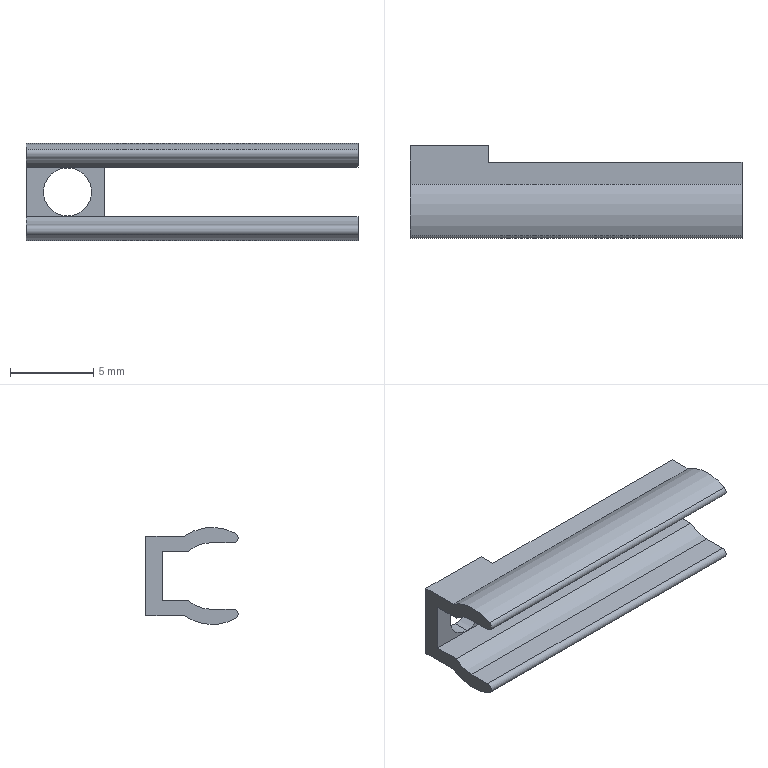Part | SolidWorks | features BaseBody 1 | 1 solid | 23 faces | box 20 x 5.565 x 5.85 mm | volume 175.472 mm3 | plane 14 | cylinder 9 | commonest cylinder face diameters 5.85 x3 0.6 x2 2.9 x2 4 x2
STEP:
#1=CARTESIAN_POINT('',(-0.5,-1.51,-2.563));
#2=VERTEX_POINT('',#1);
#3=CARTESIAN_POINT('',(-0.5,-0.1,-2.925));
#4=VERTEX_POINT('',#3);
#5=CARTESIAN_POINT('',(-0.5,-0.1,0.));
#6=DIRECTION('',(1.,0.,0.));
#7=DIRECTION('',(0.,0.,-1.));
#8=AXIS2_PLACEMENT_3D('',#5,#6,#7);
#9=CIRCLE('',#8,2.925);
#10=EDGE_CURVE('',#2,#4,#9,.T.);
#11=ORIENTED_EDGE('',*,*,#10,.T.);
#12=CARTESIAN_POINT('',(19.5,-0.1,-2.925));
#13=VERTEX_POINT('',#12);
#14=CARTESIAN_POINT('',(19.5,-0.1,-2.925));
#15=DIRECTION('',(1.,0.,0.));
#16=VECTOR('',#15,1000.);
#17=LINE('',#14,#16);
#18=EDGE_CURVE('',#4,#13,#17,.T.);
#19=ORIENTED_EDGE('',*,*,#18,.T.);
#20=CARTESIAN_POINT('',(19.5,-1.51,-2.563));
#21=VERTEX_POINT('',#20);
#22=CARTESIAN_POINT('',(19.5,-0.1,0.));
#23=DIRECTION('',(-1.,0.,0.));
#24=DIRECTION('',(0.,0.,-1.));
#25=AXIS2_PLACEMENT_3D('',#22,#23,#24);
#26=CIRCLE('',#25,2.925);
#27=EDGE_CURVE('',#13,#21,#26,.T.);
#28=ORIENTED_EDGE('',*,*,#27,.T.);
#29=CARTESIAN_POINT('',(19.5,-1.51,-2.563));
#30=DIRECTION('',(-1.,0.,0.));
#31=VECTOR('',#30,1000.);
#32=LINE('',#29,#31);
#33=EDGE_CURVE('',#21,#2,#32,.T.);
#34=ORIENTED_EDGE('',*,*,#33,.T.);
#35=EDGE_LOOP('',(#11,#19,#28,#34));
#36=FACE_OUTER_BOUND('',#35,.T.);
#37=CARTESIAN_POINT('',(19.5,-0.1,0.));
#38=DIRECTION('',(1.,0.,0.));
#39=DIRECTION('',(0.,0.,-1.));
#40=AXIS2_PLACEMENT_3D('',#37,#38,#39);
#41=CYLINDRICAL_SURFACE('',#40,2.925);
#42=ADVANCED_FACE('',(#36),#41,.T.);
#43=CARTESIAN_POINT('',(2.,2.9,1.45));
#44=VERTEX_POINT('',#43);
#45=CARTESIAN_POINT('',(2.,2.9,-1.45));
#46=VERTEX_POINT('',#45);
#47=CARTESIAN_POINT('',(2.,2.9,0.));
#48=DIRECTION('',(0.,-1.,0.));
#49=DIRECTION('',(0.,0.,1.));
#50=AXIS2_PLACEMENT_3D('',#47,#48,#49);
#51=CIRCLE('',#50,1.45);
#52=EDGE_CURVE('',#44,#46,#51,.T.);
#53=ORIENTED_EDGE('',*,*,#52,.T.);
#54=CARTESIAN_POINT('',(2.,3.9,-1.45));
#55=VERTEX_POINT('',#54);
#56=CARTESIAN_POINT('',(2.,0.,-1.45));
#57=DIRECTION('',(0.,1.,0.));
#58=VECTOR('',#57,1000.);
#59=LINE('',#56,#58);
#60=EDGE_CURVE('',#46,#55,#59,.T.);
#61=ORIENTED_EDGE('',*,*,#60,.T.);
#62=CARTESIAN_POINT('',(2.,3.9,1.45));
#63=VERTEX_POINT('',#62);
#64=CARTESIAN_POINT('',(2.,3.9,0.));
#65=DIRECTION('',(0.,1.,0.));
#66=DIRECTION('',(0.,0.,1.));
#67=AXIS2_PLACEMENT_3D('',#64,#65,#66);
#68=CIRCLE('',#67,1.45);
#69=EDGE_CURVE('',#55,#63,#68,.T.);
#70=ORIENTED_EDGE('',*,*,#69,.T.);
#71=CARTESIAN_POINT('',(2.,0.,1.45));
#72=DIRECTION('',(0.,1.,0.));
#73=VECTOR('',#72,1000.);
#74=LINE('',#71,#73);
#75=EDGE_CURVE('',#44,#63,#74,.T.);
#76=ORIENTED_EDGE('',*,*,#75,.F.);
#77=EDGE_LOOP('',(#53,#61,#70,#76));
#78=FACE_OUTER_BOUND('',#77,.T.);
#79=CARTESIAN_POINT('',(2.,0.,0.));
#80=DIRECTION('',(0.,1.,0.));
#81=DIRECTION('',(0.,0.,1.));
#82=AXIS2_PLACEMENT_3D('',#79,#80,#81);
#83=CYLINDRICAL_SURFACE('',#82,1.45);
#84=ADVANCED_FACE('',(#78),#83,.F.);
#85=ORIENTED_EDGE('',*,*,#18,.F.);
#86=CARTESIAN_POINT('',(-0.5,1.572,-2.4));
#87=VERTEX_POINT('',#86);
#88=CARTESIAN_POINT('',(-0.5,-0.1,0.));
#89=DIRECTION('',(1.,0.,0.));
#90=DIRECTION('',(0.,0.,-1.));
#91=AXIS2_PLACEMENT_3D('',#88,#89,#90);
#92=CIRCLE('',#91,2.925);
#93=EDGE_CURVE('',#4,#87,#92,.T.);
#94=ORIENTED_EDGE('',*,*,#93,.T.);
#95=CARTESIAN_POINT('',(19.5,1.572,-2.4));
#96=VERTEX_POINT('',#95);
#97=CARTESIAN_POINT('',(19.5,1.572,-2.4));
#98=DIRECTION('',(1.,0.,0.));
#99=VECTOR('',#98,1000.);
#100=LINE('',#97,#99);
#101=EDGE_CURVE('',#87,#96,#100,.T.);
#102=ORIENTED_EDGE('',*,*,#101,.T.);
#103=CARTESIAN_POINT('',(19.5,-0.1,0.));
#104=DIRECTION('',(-1.,0.,0.));
#105=DIRECTION('',(0.,0.,-1.));
#106=AXIS2_PLACEMENT_3D('',#103,#104,#105);
#107=CIRCLE('',#106,2.925);
#108=EDGE_CURVE('',#96,#13,#107,.T.);
#109=ORIENTED_EDGE('',*,*,#108,.T.);
#110=EDGE_LOOP('',(#85,#94,#102,#109));
#111=FACE_OUTER_BOUND('',#110,.T.);
#112=CARTESIAN_POINT('',(19.5,-0.1,0.));
#113=DIRECTION('',(1.,0.,0.));
#114=DIRECTION('',(0.,0.,-1.));
#115=AXIS2_PLACEMENT_3D('',#112,#113,#114);
#116=CYLINDRICAL_SURFACE('',#115,2.925);
#117=ADVANCED_FACE('',(#111),#116,.T.);
#118=CARTESIAN_POINT('',(19.5,-1.365,-2.));
#119=VERTEX_POINT('',#118);
#120=CARTESIAN_POINT('',(19.5,-1.365,-2.3));
#121=DIRECTION('',(-1.,0.,0.));
#122=DIRECTION('',(0.,0.,-1.));
#123=AXIS2_PLACEMENT_3D('',#120,#121,#122);
#124=CIRCLE('',#123,0.3);
#125=EDGE_CURVE('',#21,#119,#124,.T.);
#126=ORIENTED_EDGE('',*,*,#125,.T.);
#127=CARTESIAN_POINT('',(-0.5,-1.365,-2.));
#128=VERTEX_POINT('',#127);
#129=CARTESIAN_POINT('',(19.5,-1.365,-2.));
#130=DIRECTION('',(-1.,0.,0.));
#131=VECTOR('',#130,1000.);
#132=LINE('',#129,#131);
#133=EDGE_CURVE('',#119,#128,#132,.T.);
#134=ORIENTED_EDGE('',*,*,#133,.T.);
#135=CARTESIAN_POINT('',(-0.5,-1.365,-2.3));
#136=DIRECTION('',(1.,0.,0.));
#137=DIRECTION('',(0.,0.,-1.));
#138=AXIS2_PLACEMENT_3D('',#135,#136,#137);
#139=CIRCLE('',#138,0.3);
#140=EDGE_CURVE('',#128,#2,#139,.T.);
#141=ORIENTED_EDGE('',*,*,#140,.T.);
#142=ORIENTED_EDGE('',*,*,#33,.F.);
#143=EDGE_LOOP('',(#126,#134,#141,#142));
#144=FACE_OUTER_BOUND('',#143,.T.);
#145=CARTESIAN_POINT('',(19.5,-1.365,-2.3));
#146=DIRECTION('',(1.,0.,0.));
#147=DIRECTION('',(0.,0.,-1.));
#148=AXIS2_PLACEMENT_3D('',#145,#146,#147);
#149=CYLINDRICAL_SURFACE('',#148,0.3);
#150=ADVANCED_FACE('',(#144),#149,.T.);
#151=ORIENTED_EDGE('',*,*,#125,.F.);
#152=ORIENTED_EDGE('',*,*,#27,.F.);
#153=ORIENTED_EDGE('',*,*,#108,.F.);
#154=CARTESIAN_POINT('',(19.5,2.9,-2.4));
#155=VERTEX_POINT('',#154);
#156=CARTESIAN_POINT('',(19.5,-0.1,-2.4));
#157=DIRECTION('',(0.,1.,0.));
#158=VECTOR('',#157,1000.);
#159=LINE('',#156,#158);
#160=EDGE_CURVE('',#96,#155,#159,.T.);
#161=ORIENTED_EDGE('',*,*,#160,.T.);
#162=CARTESIAN_POINT('',(19.5,2.9,-1.5));
#163=VERTEX_POINT('',#162);
#164=CARTESIAN_POINT('',(19.5,2.9,2.4));
#165=DIRECTION('',(0.,0.,-1.));
#166=VECTOR('',#165,1000.);
#167=LINE('',#164,#166);
#168=EDGE_CURVE('',#163,#155,#167,.T.);
#169=ORIENTED_EDGE('',*,*,#168,.F.);
#170=CARTESIAN_POINT('',(19.5,1.323,-1.5));
#171=VERTEX_POINT('',#170);
#172=CARTESIAN_POINT('',(19.5,2.9,-1.5));
#173=DIRECTION('',(0.,-1.,0.));
#174=VECTOR('',#173,1000.);
#175=LINE('',#172,#174);
#176=EDGE_CURVE('',#163,#171,#175,.T.);
#177=ORIENTED_EDGE('',*,*,#176,.T.);
#178=CARTESIAN_POINT('',(19.5,0.,-2.));
#179=VERTEX_POINT('',#178);
#180=CARTESIAN_POINT('',(19.5,0.,0.));
#181=DIRECTION('',(-1.,0.,0.));
#182=DIRECTION('',(0.,0.,-1.));
#183=AXIS2_PLACEMENT_3D('',#180,#181,#182);
#184=CIRCLE('',#183,2.);
#185=EDGE_CURVE('',#171,#179,#184,.T.);
#186=ORIENTED_EDGE('',*,*,#185,.T.);
#187=CARTESIAN_POINT('',(19.5,-0.1,-2.));
#188=DIRECTION('',(0.,-1.,0.));
#189=VECTOR('',#188,1000.);
#190=LINE('',#187,#189);
#191=EDGE_CURVE('',#179,#119,#190,.T.);
#192=ORIENTED_EDGE('',*,*,#191,.T.);
#193=EDGE_LOOP('',(#151,#152,#153,#161,#169,#177,#186,#192));
#194=FACE_OUTER_BOUND('',#193,.T.);
#195=CARTESIAN_POINT('',(19.5,-0.1,0.));
#196=DIRECTION('',(1.,0.,0.));
#197=DIRECTION('',(0.,0.,-1.));
#198=AXIS2_PLACEMENT_3D('',#195,#196,#197);
#199=PLANE('',#198);
#200=ADVANCED_FACE('',(#194),#199,.T.);
#201=ORIENTED_EDGE('',*,*,#160,.F.);
#202=ORIENTED_EDGE('',*,*,#101,.F.);
#203=CARTESIAN_POINT('',(-0.5,3.9,-2.4));
#204=VERTEX_POINT('',#203);
#205=CARTESIAN_POINT('',(-0.5,1.572,-2.4));
#206=DIRECTION('',(0.,-1.,0.));
#207=VECTOR('',#206,1000.);
#208=LINE('',#205,#207);
#209=EDGE_CURVE('',#204,#87,#208,.T.);
#210=ORIENTED_EDGE('',*,*,#209,.F.);
#211=CARTESIAN_POINT('',(4.2,3.9,-2.4));
#212=VERTEX_POINT('',#211);
#213=CARTESIAN_POINT('',(19.5,3.9,-2.4));
#214=DIRECTION('',(-1.,0.,0.));
#215=VECTOR('',#214,1000.);
#216=LINE('',#213,#215);
#217=EDGE_CURVE('',#212,#204,#216,.T.);
#218=ORIENTED_EDGE('',*,*,#217,.F.);
#219=CARTESIAN_POINT('',(4.2,2.9,-2.4));
#220=VERTEX_POINT('',#219);
#221=CARTESIAN_POINT('',(4.2,0.,-2.4));
#222=DIRECTION('',(0.,1.,0.));
#223=VECTOR('',#222,1000.);
#224=LINE('',#221,#223);
#225=EDGE_CURVE('',#220,#212,#224,.T.);
#226=ORIENTED_EDGE('',*,*,#225,.F.);
#227=CARTESIAN_POINT('',(19.5,2.9,-2.4));
#228=DIRECTION('',(-1.,0.,0.));
#229=VECTOR('',#228,1000.);
#230=LINE('',#227,#229);
#231=EDGE_CURVE('',#155,#220,#230,.T.);
#232=ORIENTED_EDGE('',*,*,#231,.F.);
#233=EDGE_LOOP('',(#201,#202,#210,#218,#226,#232));
#234=FACE_OUTER_BOUND('',#233,.T.);
#235=CARTESIAN_POINT('',(19.5,1.572,-2.4));
#236=DIRECTION('',(0.,0.,1.));
#237=DIRECTION('',(1.,0.,0.));
#238=AXIS2_PLACEMENT_3D('',#235,#236,#237);
#239=PLANE('',#238);
#240=ADVANCED_FACE('',(#234),#239,.F.);
#241=CARTESIAN_POINT('',(-0.5,3.9,2.4));
#242=VERTEX_POINT('',#241);
#243=CARTESIAN_POINT('',(-0.5,3.9,0.));
#244=DIRECTION('',(0.,0.,1.));
#245=VECTOR('',#244,1000.);
#246=LINE('',#243,#245);
#247=EDGE_CURVE('',#204,#242,#246,.T.);
#248=ORIENTED_EDGE('',*,*,#247,.F.);
#249=ORIENTED_EDGE('',*,*,#209,.T.);
#250=ORIENTED_EDGE('',*,*,#93,.F.);
#251=ORIENTED_EDGE('',*,*,#10,.F.);
#252=ORIENTED_EDGE('',*,*,#140,.F.);
#253=CARTESIAN_POINT('',(-0.5,0.,-2.));
#254=VERTEX_POINT('',#253);
#255=CARTESIAN_POINT('',(-0.5,-0.1,-2.));
#256=DIRECTION('',(0.,-1.,0.));
#257=VECTOR('',#256,1000.);
#258=LINE('',#255,#257);
#259=EDGE_CURVE('',#254,#128,#258,.T.);
#260=ORIENTED_EDGE('',*,*,#259,.F.);
#261=CARTESIAN_POINT('',(-0.5,1.323,-1.5));
#262=VERTEX_POINT('',#261);
#263=CARTESIAN_POINT('',(-0.5,0.,0.));
#264=DIRECTION('',(1.,0.,0.));
#265=DIRECTION('',(0.,0.,-1.));
#266=AXIS2_PLACEMENT_3D('',#263,#264,#265);
#267=CIRCLE('',#266,2.);
#268=EDGE_CURVE('',#254,#262,#267,.T.);
#269=ORIENTED_EDGE('',*,*,#268,.T.);
#270=CARTESIAN_POINT('',(-0.5,2.9,-1.5));
#271=VERTEX_POINT('',#270);
#272=CARTESIAN_POINT('',(-0.5,2.9,-1.5));
#273=DIRECTION('',(0.,1.,0.));
#274=VECTOR('',#273,1000.);
#275=LINE('',#272,#274);
#276=EDGE_CURVE('',#262,#271,#275,.T.);
#277=ORIENTED_EDGE('',*,*,#276,.T.);
#278=CARTESIAN_POINT('',(-0.5,2.9,1.5));
#279=VERTEX_POINT('',#278);
#280=CARTESIAN_POINT('',(-0.5,2.9,0.));
#281=DIRECTION('',(0.,0.,-1.));
#282=VECTOR('',#281,1000.);
#283=LINE('',#280,#282);
#284=EDGE_CURVE('',#279,#271,#283,.T.);
#285=ORIENTED_EDGE('',*,*,#284,.F.);
#286=CARTESIAN_POINT('',(-0.5,1.323,1.5));
#287=VERTEX_POINT('',#286);
#288=CARTESIAN_POINT('',(-0.5,1.323,1.5));
#289=DIRECTION('',(0.,-1.,0.));
#290=VECTOR('',#289,1000.);
#291=LINE('',#288,#290);
#292=EDGE_CURVE('',#279,#287,#291,.T.);
#293=ORIENTED_EDGE('',*,*,#292,.T.);
#294=CARTESIAN_POINT('',(-0.5,0.,2.));
#295=VERTEX_POINT('',#294);
#296=CARTESIAN_POINT('',(-0.5,0.,0.));
#297=DIRECTION('',(1.,0.,0.));
#298=DIRECTION('',(0.,0.,-1.));
#299=AXIS2_PLACEMENT_3D('',#296,#297,#298);
#300=CIRCLE('',#299,2.);
#301=EDGE_CURVE('',#287,#295,#300,.T.);
#302=ORIENTED_EDGE('',*,*,#301,.T.);
#303=CARTESIAN_POINT('',(-0.5,-1.365,2.));
#304=VERTEX_POINT('',#303);
#305=CARTESIAN_POINT('',(-0.5,-1.365,2.));
#306=DIRECTION('',(0.,-1.,0.));
#307=VECTOR('',#306,1000.);
#308=LINE('',#305,#307);
#309=EDGE_CURVE('',#295,#304,#308,.T.);
#310=ORIENTED_EDGE('',*,*,#309,.T.);
#311=CARTESIAN_POINT('',(-0.5,-1.51,2.563));
#312=VERTEX_POINT('',#311);
#313=CARTESIAN_POINT('',(-0.5,-1.365,2.3));
#314=DIRECTION('',(1.,0.,0.));
#315=DIRECTION('',(0.,0.,-1.));
#316=AXIS2_PLACEMENT_3D('',#313,#314,#315);
#317=CIRCLE('',#316,0.3);
#318=EDGE_CURVE('',#312,#304,#317,.T.);
#319=ORIENTED_EDGE('',*,*,#318,.F.);
#320=CARTESIAN_POINT('',(-0.5,1.572,2.4));
#321=VERTEX_POINT('',#320);
#322=CARTESIAN_POINT('',(-0.5,-0.1,0.));
#323=DIRECTION('',(1.,0.,0.));
#324=DIRECTION('',(0.,0.,-1.));
#325=AXIS2_PLACEMENT_3D('',#322,#323,#324);
#326=CIRCLE('',#325,2.925);
#327=EDGE_CURVE('',#321,#312,#326,.T.);
#328=ORIENTED_EDGE('',*,*,#327,.F.);
#329=CARTESIAN_POINT('',(-0.5,-0.1,2.4));
#330=DIRECTION('',(0.,-1.,0.));
#331=VECTOR('',#330,1000.);
#332=LINE('',#329,#331);
#333=EDGE_CURVE('',#242,#321,#332,.T.);
#334=ORIENTED_EDGE('',*,*,#333,.F.);
#335=EDGE_LOOP('',(#248,#249,#250,#251,#252,#260,#269,#277,#285,#293,#302,#310,#319,#328,#334));
#336=FACE_OUTER_BOUND('',#335,.T.);
#337=CARTESIAN_POINT('',(-0.5,-0.1,0.));
#338=DIRECTION('',(1.,0.,0.));
#339=DIRECTION('',(0.,0.,-1.));
#340=AXIS2_PLACEMENT_3D('',#337,#338,#339);
#341=PLANE('',#340);
#342=ADVANCED_FACE('',(#336),#341,.F.);
#343=ORIENTED_EDGE('',*,*,#133,.F.);
#344=ORIENTED_EDGE('',*,*,#191,.F.);
#345=CARTESIAN_POINT('',(19.5,0.,-2.));
#346=DIRECTION('',(1.,0.,0.));
#347=VECTOR('',#346,1000.);
#348=LINE('',#345,#347);
#349=EDGE_CURVE('',#254,#179,#348,.T.);
#350=ORIENTED_EDGE('',*,*,#349,.F.);
#351=ORIENTED_EDGE('',*,*,#259,.T.);
#352=EDGE_LOOP('',(#343,#344,#350,#351));
#353=FACE_OUTER_BOUND('',#352,.T.);
#354=CARTESIAN_POINT('',(19.5,0.,-2.));
#355=DIRECTION('',(0.,0.,-1.));
#356=DIRECTION('',(-1.,0.,0.));
#357=AXIS2_PLACEMENT_3D('',#354,#355,#356);
#358=PLANE('',#357);
#359=ADVANCED_FACE('',(#353),#358,.F.);
#360=ORIENTED_EDGE('',*,*,#231,.T.);
#361=CARTESIAN_POINT('',(4.2,2.9,-1.5));
#362=VERTEX_POINT('',#361);
#363=CARTESIAN_POINT('',(4.2,2.9,0.));
#364=DIRECTION('',(0.,0.,-1.));
#365=VECTOR('',#364,1000.);
#366=LINE('',#363,#365);
#367=EDGE_CURVE('',#362,#220,#366,.T.);
#368=ORIENTED_EDGE('',*,*,#367,.F.);
#369=CARTESIAN_POINT('',(22.2,2.9,-1.5));
#370=DIRECTION('',(1.,0.,0.));
#371=VECTOR('',#370,1000.);
#372=LINE('',#369,#371);
#373=EDGE_CURVE('',#362,#163,#372,.T.);
#374=ORIENTED_EDGE('',*,*,#373,.T.);
#375=ORIENTED_EDGE('',*,*,#168,.T.);
#376=EDGE_LOOP('',(#360,#368,#374,#375));
#377=FACE_OUTER_BOUND('',#376,.T.);
#378=CARTESIAN_POINT('',(22.2,2.9,2.4));
#379=DIRECTION('',(0.,1.,0.));
#380=DIRECTION('',(0.,0.,1.));
#381=AXIS2_PLACEMENT_3D('',#378,#379,#380);
#382=PLANE('',#381);
#383=ADVANCED_FACE('',(#377),#382,.T.);
#384=ORIENTED_EDGE('',*,*,#217,.T.);
#385=ORIENTED_EDGE('',*,*,#247,.T.);
#386=CARTESIAN_POINT('',(4.2,3.9,2.4));
#387=VERTEX_POINT('',#386);
#388=CARTESIAN_POINT('',(19.5,3.9,2.4));
#389=DIRECTION('',(-1.,0.,0.));
#390=VECTOR('',#389,1000.);
#391=LINE('',#388,#390);
#392=EDGE_CURVE('',#387,#242,#391,.T.);
#393=ORIENTED_EDGE('',*,*,#392,.F.);
#394=CARTESIAN_POINT('',(4.2,3.9,-2.4));
#395=DIRECTION('',(0.,0.,1.));
#396=VECTOR('',#395,1000.);
#397=LINE('',#394,#396);
#398=EDGE_CURVE('',#212,#387,#397,.T.);
#399=ORIENTED_EDGE('',*,*,#398,.F.);
#400=EDGE_LOOP('',(#384,#385,#393,#399));
#401=FACE_OUTER_BOUND('',#400,.T.);
#402=CARTESIAN_POINT('',(2.,3.9,0.));
#403=DIRECTION('',(0.,1.,0.));
#404=DIRECTION('',(0.,0.,1.));
#405=AXIS2_PLACEMENT_3D('',#402,#403,#404);
#406=CIRCLE('',#405,1.45);
#407=EDGE_CURVE('',#63,#55,#406,.T.);
#408=ORIENTED_EDGE('',*,*,#407,.F.);
#409=ORIENTED_EDGE('',*,*,#69,.F.);
#410=EDGE_LOOP('',(#408,#409));
#411=FACE_BOUND('',#410,.T.);
#412=CARTESIAN_POINT('',(19.5,3.9,-2.4));
#413=DIRECTION('',(0.,-1.,0.));
#414=DIRECTION('',(0.,0.,-1.));
#415=AXIS2_PLACEMENT_3D('',#412,#413,#414);
#416=PLANE('',#415);
#417=ADVANCED_FACE('',(#401,#411),#416,.F.);
#418=CARTESIAN_POINT('',(4.2,2.9,2.4));
#419=VERTEX_POINT('',#418);
#420=CARTESIAN_POINT('',(4.2,3.9,2.4));
#421=DIRECTION('',(0.,-1.,0.));
#422=VECTOR('',#421,1000.);
#423=LINE('',#420,#422);
#424=EDGE_CURVE('',#387,#419,#423,.T.);
#425=ORIENTED_EDGE('',*,*,#424,.F.);
#426=ORIENTED_EDGE('',*,*,#392,.T.);
#427=ORIENTED_EDGE('',*,*,#333,.T.);
#428=CARTESIAN_POINT('',(19.5,1.572,2.4));
#429=VERTEX_POINT('',#428);
#430=CARTESIAN_POINT('',(19.5,1.572,2.4));
#431=DIRECTION('',(-1.,0.,0.));
#432=VECTOR('',#431,1000.);
#433=LINE('',#430,#432);
#434=EDGE_CURVE('',#429,#321,#433,.T.);
#435=ORIENTED_EDGE('',*,*,#434,.F.);
#436=CARTESIAN_POINT('',(19.5,2.9,2.4));
#437=VERTEX_POINT('',#436);
#438=CARTESIAN_POINT('',(19.5,-0.1,2.4));
#439=DIRECTION('',(0.,-1.,0.));
#440=VECTOR('',#439,1000.);
#441=LINE('',#438,#440);
#442=EDGE_CURVE('',#437,#429,#441,.T.);
#443=ORIENTED_EDGE('',*,*,#442,.F.);
#444=CARTESIAN_POINT('',(19.5,2.9,2.4));
#445=DIRECTION('',(1.,0.,0.));
#446=VECTOR('',#445,1000.);
#447=LINE('',#444,#446);
#448=EDGE_CURVE('',#419,#437,#447,.T.);
#449=ORIENTED_EDGE('',*,*,#448,.F.);
#450=EDGE_LOOP('',(#425,#426,#427,#435,#443,#449));
#451=FACE_OUTER_BOUND('',#450,.T.);
#452=CARTESIAN_POINT('',(19.5,3.9,2.4));
#453=DIRECTION('',(0.,0.,-1.));
#454=DIRECTION('',(-1.,0.,0.));
#455=AXIS2_PLACEMENT_3D('',#452,#453,#454);
#456=PLANE('',#455);
#457=ADVANCED_FACE('',(#451),#456,.F.);
#458=CARTESIAN_POINT('',(4.2,2.9,1.5));
#459=VERTEX_POINT('',#458);
#460=CARTESIAN_POINT('',(19.5,2.9,1.5));
#461=DIRECTION('',(1.,0.,0.));
#462=VECTOR('',#461,1000.);
#463=LINE('',#460,#462);
#464=EDGE_CURVE('',#279,#459,#463,.T.);
#465=ORIENTED_EDGE('',*,*,#464,.F.);
#466=ORIENTED_EDGE('',*,*,#284,.T.);
#467=CARTESIAN_POINT('',(19.5,2.9,-1.5));
#468=DIRECTION('',(-1.,0.,0.));
#469=VECTOR('',#468,1000.);
#470=LINE('',#467,#469);
#471=EDGE_CURVE('',#362,#271,#470,.T.);
#472=ORIENTED_EDGE('',*,*,#471,.F.);
#473=CARTESIAN_POINT('',(4.2,2.9,1.5));
#474=DIRECTION('',(0.,0.,-1.));
#475=VECTOR('',#474,1000.);
#476=LINE('',#473,#475);
#477=EDGE_CURVE('',#459,#362,#476,.T.);
#478=ORIENTED_EDGE('',*,*,#477,.F.);
#479=EDGE_LOOP('',(#465,#466,#472,#478));
#480=FACE_OUTER_BOUND('',#479,.T.);
#481=ORIENTED_EDGE('',*,*,#52,.F.);
#482=CARTESIAN_POINT('',(2.,2.9,0.));
#483=DIRECTION('',(0.,-1.,0.));
#484=DIRECTION('',(0.,0.,1.));
#485=AXIS2_PLACEMENT_3D('',#482,#483,#484);
#486=CIRCLE('',#485,1.45);
#487=EDGE_CURVE('',#46,#44,#486,.T.);
#488=ORIENTED_EDGE('',*,*,#487,.F.);
#489=EDGE_LOOP('',(#481,#488));
#490=FACE_BOUND('',#489,.T.);
#491=CARTESIAN_POINT('',(19.5,2.9,1.5));
#492=DIRECTION('',(0.,1.,0.));
#493=DIRECTION('',(0.,0.,1.));
#494=AXIS2_PLACEMENT_3D('',#491,#492,#493);
#495=PLANE('',#494);
#496=ADVANCED_FACE('',(#480,#490),#495,.F.);
#497=CARTESIAN_POINT('',(19.5,-1.51,2.563));
#498=VERTEX_POINT('',#497);
#499=CARTESIAN_POINT('',(19.5,-0.1,0.));
#500=DIRECTION('',(-1.,0.,0.));
#501=DIRECTION('',(0.,0.,-1.));
#502=AXIS2_PLACEMENT_3D('',#499,#500,#501);
#503=CIRCLE('',#502,2.925);
#504=EDGE_CURVE('',#498,#429,#503,.T.);
#505=ORIENTED_EDGE('',*,*,#504,.T.);
#506=ORIENTED_EDGE('',*,*,#434,.T.);
#507=ORIENTED_EDGE('',*,*,#327,.T.);
#508=CARTESIAN_POINT('',(19.5,-1.51,2.563));
#509=DIRECTION('',(1.,0.,0.));
#510=VECTOR('',#509,1000.);
#511=LINE('',#508,#510);
#512=EDGE_CURVE('',#312,#498,#511,.T.);
#513=ORIENTED_EDGE('',*,*,#512,.T.);
#514=EDGE_LOOP('',(#505,#506,#507,#513));
#515=FACE_OUTER_BOUND('',#514,.T.);
#516=CARTESIAN_POINT('',(19.5,-0.1,0.));
#517=DIRECTION('',(1.,0.,0.));
#518=DIRECTION('',(0.,0.,-1.));
#519=AXIS2_PLACEMENT_3D('',#516,#517,#518);
#520=CYLINDRICAL_SURFACE('',#519,2.925);
#521=ADVANCED_FACE('',(#515),#520,.T.);
#522=ORIENTED_EDGE('',*,*,#349,.T.);
#523=ORIENTED_EDGE('',*,*,#185,.F.);
#524=CARTESIAN_POINT('',(19.5,1.323,-1.5));
#525=DIRECTION('',(1.,0.,0.));
#526=VECTOR('',#525,1000.);
#527=LINE('',#524,#526);
#528=EDGE_CURVE('',#262,#171,#527,.T.);
#529=ORIENTED_EDGE('',*,*,#528,.F.);
#530=ORIENTED_EDGE('',*,*,#268,.F.);
#531=EDGE_LOOP('',(#522,#523,#529,#530));
#532=FACE_OUTER_BOUND('',#531,.T.);
#533=CARTESIAN_POINT('',(19.5,0.,0.));
#534=DIRECTION('',(1.,0.,0.));
#535=DIRECTION('',(0.,0.,-1.));
#536=AXIS2_PLACEMENT_3D('',#533,#534,#535);
#537=CYLINDRICAL_SURFACE('',#536,2.);
#538=ADVANCED_FACE('',(#532),#537,.F.);
#539=ORIENTED_EDGE('',*,*,#528,.T.);
#540=ORIENTED_EDGE('',*,*,#176,.F.);
#541=ORIENTED_EDGE('',*,*,#373,.F.);
#542=ORIENTED_EDGE('',*,*,#471,.T.);
#543=ORIENTED_EDGE('',*,*,#276,.F.);
#544=EDGE_LOOP('',(#539,#540,#541,#542,#543));
#545=FACE_OUTER_BOUND('',#544,.T.);
#546=CARTESIAN_POINT('',(19.5,2.9,-1.5));
#547=DIRECTION('',(0.,0.,-1.));
#548=DIRECTION('',(-1.,0.,0.));
#549=AXIS2_PLACEMENT_3D('',#546,#547,#548);
#550=PLANE('',#549);
#551=ADVANCED_FACE('',(#545),#550,.F.);
#552=ORIENTED_EDGE('',*,*,#225,.T.);
#553=ORIENTED_EDGE('',*,*,#398,.T.);
#554=ORIENTED_EDGE('',*,*,#424,.T.);
#555=CARTESIAN_POINT('',(4.2,2.9,0.));
#556=DIRECTION('',(0.,0.,-1.));
#557=VECTOR('',#556,1000.);
#558=LINE('',#555,#557);
#559=EDGE_CURVE('',#419,#459,#558,.T.);
#560=ORIENTED_EDGE('',*,*,#559,.T.);
#561=ORIENTED_EDGE('',*,*,#477,.T.);
#562=ORIENTED_EDGE('',*,*,#367,.T.);
#563=EDGE_LOOP('',(#552,#553,#554,#560,#561,#562));
#564=FACE_OUTER_BOUND('',#563,.T.);
#565=CARTESIAN_POINT('',(4.2,0.,0.));
#566=DIRECTION('',(1.,0.,0.));
#567=DIRECTION('',(0.,0.,-1.));
#568=AXIS2_PLACEMENT_3D('',#565,#566,#567);
#569=PLANE('',#568);
#570=ADVANCED_FACE('',(#564),#569,.T.);
#571=ORIENTED_EDGE('',*,*,#60,.F.);
#572=ORIENTED_EDGE('',*,*,#487,.T.);
#573=ORIENTED_EDGE('',*,*,#75,.T.);
#574=ORIENTED_EDGE('',*,*,#407,.T.);
#575=EDGE_LOOP('',(#571,#572,#573,#574));
#576=FACE_OUTER_BOUND('',#575,.T.);
#577=CARTESIAN_POINT('',(2.,0.,0.));
#578=DIRECTION('',(0.,1.,0.));
#579=DIRECTION('',(0.,0.,1.));
#580=AXIS2_PLACEMENT_3D('',#577,#578,#579);
#581=CYLINDRICAL_SURFACE('',#580,1.45);
#582=ADVANCED_FACE('',(#576),#581,.F.);
#583=ORIENTED_EDGE('',*,*,#448,.T.);
#584=CARTESIAN_POINT('',(19.5,2.9,1.5));
#585=VERTEX_POINT('',#584);
#586=CARTESIAN_POINT('',(19.5,2.9,2.4));
#587=DIRECTION('',(0.,0.,-1.));
#588=VECTOR('',#587,1000.);
#589=LINE('',#586,#588);
#590=EDGE_CURVE('',#437,#585,#589,.T.);
#591=ORIENTED_EDGE('',*,*,#590,.T.);
#592=CARTESIAN_POINT('',(22.2,2.9,1.5));
#593=DIRECTION('',(-1.,0.,0.));
#594=VECTOR('',#593,1000.);
#595=LINE('',#592,#594);
#596=EDGE_CURVE('',#585,#459,#595,.T.);
#597=ORIENTED_EDGE('',*,*,#596,.T.);
#598=ORIENTED_EDGE('',*,*,#559,.F.);
#599=EDGE_LOOP('',(#583,#591,#597,#598));
#600=FACE_OUTER_BOUND('',#599,.T.);
#601=CARTESIAN_POINT('',(22.2,2.9,2.4));
#602=DIRECTION('',(0.,1.,0.));
#603=DIRECTION('',(0.,0.,1.));
#604=AXIS2_PLACEMENT_3D('',#601,#602,#603);
#605=PLANE('',#604);
#606=ADVANCED_FACE('',(#600),#605,.T.);
#607=ORIENTED_EDGE('',*,*,#464,.T.);
#608=ORIENTED_EDGE('',*,*,#596,.F.);
#609=CARTESIAN_POINT('',(19.5,1.323,1.5));
#610=VERTEX_POINT('',#609);
#611=CARTESIAN_POINT('',(19.5,1.323,1.5));
#612=DIRECTION('',(0.,1.,0.));
#613=VECTOR('',#612,1000.);
#614=LINE('',#611,#613);
#615=EDGE_CURVE('',#610,#585,#614,.T.);
#616=ORIENTED_EDGE('',*,*,#615,.F.);
#617=CARTESIAN_POINT('',(19.5,1.323,1.5));
#618=DIRECTION('',(1.,0.,0.));
#619=VECTOR('',#618,1000.);
#620=LINE('',#617,#619);
#621=EDGE_CURVE('',#287,#610,#620,.T.);
#622=ORIENTED_EDGE('',*,*,#621,.F.);
#623=ORIENTED_EDGE('',*,*,#292,.F.);
#624=EDGE_LOOP('',(#607,#608,#616,#622,#623));
#625=FACE_OUTER_BOUND('',#624,.T.);
#626=CARTESIAN_POINT('',(19.5,1.323,1.5));
#627=DIRECTION('',(0.,0.,1.));
#628=DIRECTION('',(1.,0.,0.));
#629=AXIS2_PLACEMENT_3D('',#626,#627,#628);
#630=PLANE('',#629);
#631=ADVANCED_FACE('',(#625),#630,.F.);
#632=CARTESIAN_POINT('',(19.5,-1.365,2.));
#633=VERTEX_POINT('',#632);
#634=CARTESIAN_POINT('',(19.5,0.,2.));
#635=VERTEX_POINT('',#634);
#636=CARTESIAN_POINT('',(19.5,-1.365,2.));
#637=DIRECTION('',(0.,1.,0.));
#638=VECTOR('',#637,1000.);
#639=LINE('',#636,#638);
#640=EDGE_CURVE('',#633,#635,#639,.T.);
#641=ORIENTED_EDGE('',*,*,#640,.T.);
#642=CARTESIAN_POINT('',(19.5,0.,0.));
#643=DIRECTION('',(-1.,0.,0.));
#644=DIRECTION('',(0.,0.,-1.));
#645=AXIS2_PLACEMENT_3D('',#642,#643,#644);
#646=CIRCLE('',#645,2.);
#647=EDGE_CURVE('',#635,#610,#646,.T.);
#648=ORIENTED_EDGE('',*,*,#647,.T.);
#649=ORIENTED_EDGE('',*,*,#615,.T.);
#650=ORIENTED_EDGE('',*,*,#590,.F.);
#651=ORIENTED_EDGE('',*,*,#442,.T.);
#652=ORIENTED_EDGE('',*,*,#504,.F.);
#653=CARTESIAN_POINT('',(19.5,-1.365,2.3));
#654=DIRECTION('',(1.,0.,0.));
#655=DIRECTION('',(0.,0.,-1.));
#656=AXIS2_PLACEMENT_3D('',#653,#654,#655);
#657=CIRCLE('',#656,0.3);
#658=EDGE_CURVE('',#498,#633,#657,.T.);
#659=ORIENTED_EDGE('',*,*,#658,.T.);
#660=EDGE_LOOP('',(#641,#648,#649,#650,#651,#652,#659));
#661=FACE_OUTER_BOUND('',#660,.T.);
#662=CARTESIAN_POINT('',(19.5,-0.1,0.));
#663=DIRECTION('',(1.,0.,0.));
#664=DIRECTION('',(0.,0.,-1.));
#665=AXIS2_PLACEMENT_3D('',#662,#663,#664);
#666=PLANE('',#665);
#667=ADVANCED_FACE('',(#661),#666,.T.);
#668=ORIENTED_EDGE('',*,*,#658,.F.);
#669=ORIENTED_EDGE('',*,*,#512,.F.);
#670=ORIENTED_EDGE('',*,*,#318,.T.);
#671=CARTESIAN_POINT('',(19.5,-1.365,2.));
#672=DIRECTION('',(1.,0.,0.));
#673=VECTOR('',#672,1000.);
#674=LINE('',#671,#673);
#675=EDGE_CURVE('',#304,#633,#674,.T.);
#676=ORIENTED_EDGE('',*,*,#675,.T.);
#677=EDGE_LOOP('',(#668,#669,#670,#676));
#678=FACE_OUTER_BOUND('',#677,.T.);
#679=CARTESIAN_POINT('',(19.5,-1.365,2.3));
#680=DIRECTION('',(1.,0.,0.));
#681=DIRECTION('',(0.,0.,-1.));
#682=AXIS2_PLACEMENT_3D('',#679,#680,#681);
#683=CYLINDRICAL_SURFACE('',#682,0.3);
#684=ADVANCED_FACE('',(#678),#683,.T.);
#685=ORIENTED_EDGE('',*,*,#621,.T.);
#686=ORIENTED_EDGE('',*,*,#647,.F.);
#687=CARTESIAN_POINT('',(19.5,0.,2.));
#688=DIRECTION('',(1.,0.,0.));
#689=VECTOR('',#688,1000.);
#690=LINE('',#687,#689);
#691=EDGE_CURVE('',#295,#635,#690,.T.);
#692=ORIENTED_EDGE('',*,*,#691,.F.);
#693=ORIENTED_EDGE('',*,*,#301,.F.);
#694=EDGE_LOOP('',(#685,#686,#692,#693));
#695=FACE_OUTER_BOUND('',#694,.T.);
#696=CARTESIAN_POINT('',(19.5,0.,0.));
#697=DIRECTION('',(1.,0.,0.));
#698=DIRECTION('',(0.,0.,-1.));
#699=AXIS2_PLACEMENT_3D('',#696,#697,#698);
#700=CYLINDRICAL_SURFACE('',#699,2.);
#701=ADVANCED_FACE('',(#695),#700,.F.);
#702=ORIENTED_EDGE('',*,*,#691,.T.);
#703=ORIENTED_EDGE('',*,*,#640,.F.);
#704=ORIENTED_EDGE('',*,*,#675,.F.);
#705=ORIENTED_EDGE('',*,*,#309,.F.);
#706=EDGE_LOOP('',(#702,#703,#704,#705));
#707=FACE_OUTER_BOUND('',#706,.T.);
#708=CARTESIAN_POINT('',(19.5,-1.365,2.));
#709=DIRECTION('',(0.,0.,1.));
#710=DIRECTION('',(1.,0.,0.));
#711=AXIS2_PLACEMENT_3D('',#708,#709,#710);
#712=PLANE('',#711);
#713=ADVANCED_FACE('',(#707),#712,.F.);
#714=CLOSED_SHELL('',(#42,#84,#117,#150,#200,#240,#342,#359,#383,#417,#457,#496,#521,#538,#551,#570,#582,#606,#631,#667,#684,#701,#713));
#715=MANIFOLD_SOLID_BREP('',#714);
#716=CARTESIAN_POINT('',(0.,0.,0.));
#717=DIRECTION('',(0.,0.,1.));
#718=DIRECTION('',(1.,0.,0.));
#719=AXIS2_PLACEMENT_3D('',#716,#717,#718);
#720=(LENGTH_UNIT()NAMED_UNIT(*)SI_UNIT(.MILLI.,.METRE.));
#721=UNCERTAINTY_MEASURE_WITH_UNIT(LENGTH_MEASURE(0.00001),#720,'','');
#722=(NAMED_UNIT(*)PLANE_ANGLE_UNIT()SI_UNIT($,.RADIAN.));
#723=(NAMED_UNIT(*)SI_UNIT($,.STERADIAN.)SOLID_ANGLE_UNIT());
#724=(GEOMETRIC_REPRESENTATION_CONTEXT(3)GLOBAL_UNCERTAINTY_ASSIGNED_CONTEXT((#721))GLOBAL_UNIT_ASSIGNED_CONTEXT((#720,#722,#723))REPRESENTATION_CONTEXT('',''));
#725=ADVANCED_BREP_SHAPE_REPRESENTATION('',(#715,#719),#724);